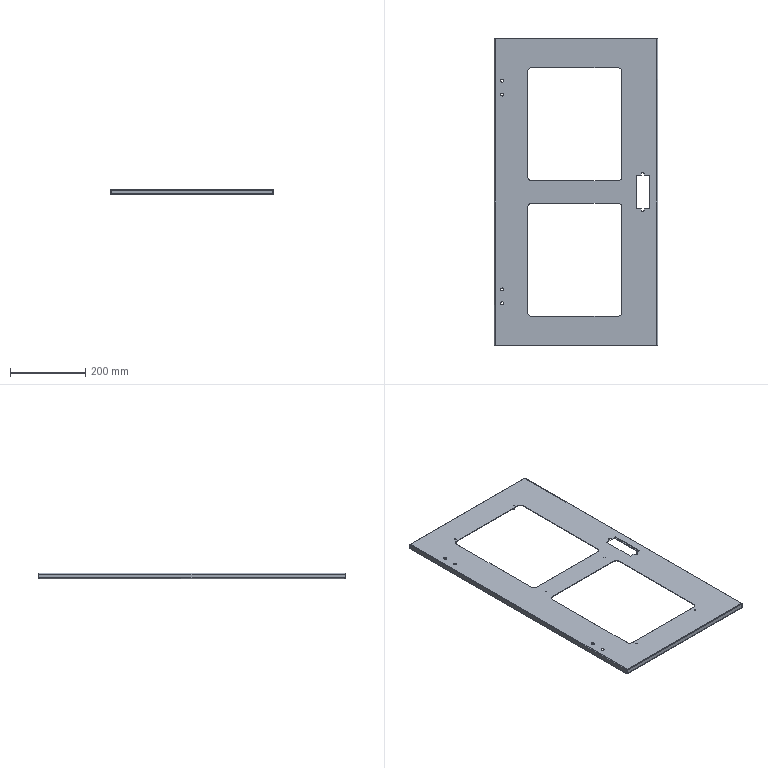Part | STEP file | 09-12 upper door A (Default) | 1 solid | 124 faces | box 434 x 818 x 15 mm | volume 398163 mm3 | plane 62 | cylinder 46 | spline 16 | commonest cylinder face diameters 4 x12 8 x10 1.473 x8 4.473 x8 20 x8